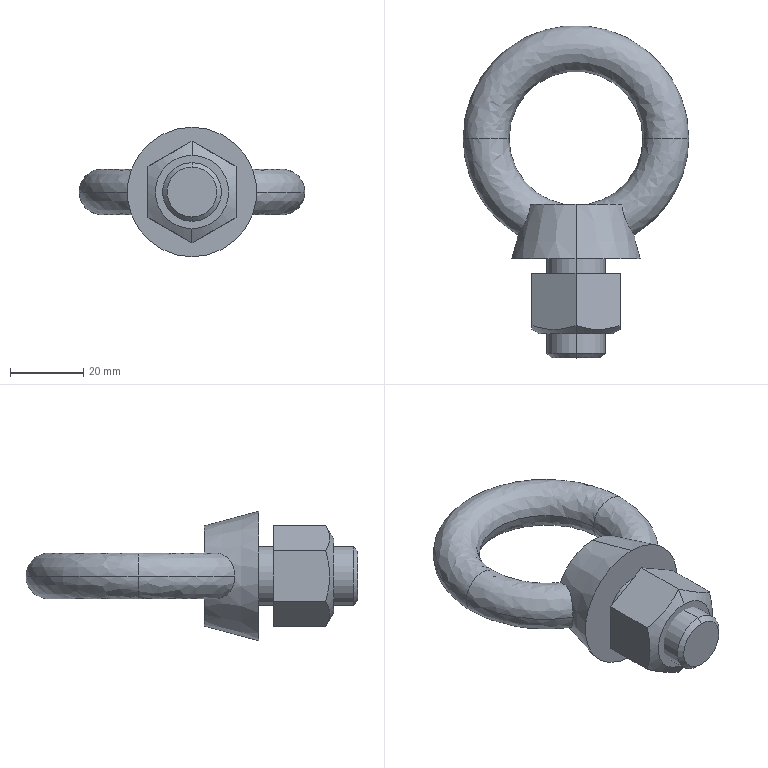Part | STEP file | M16-Lifting eye | 2 solids | 31 faces | box 61.5 x 90.6 x 35.3 mm | volume 37230 mm3 | plane 11 | cone 10 | spline 6 | cylinder 4 | commonest cylinder face diameters 16 x4
STEP:
#1=CARTESIAN_POINT('',(18.25,36.85,0.));
#2=VERTEX_POINT('',#1);
#3=CARTESIAN_POINT('',(3.295,18.9,0.));
#4=VERTEX_POINT('',#3);
#5=CARTESIAN_POINT('',(0.,36.85,0.));
#6=DIRECTION('',(0.,0.,-1.));
#7=DIRECTION('',(-1.,0.,0.));
#8=AXIS2_PLACEMENT_3D('',#5,#6,#7);
#9=CIRCLE('',#8,18.25);
#10=EDGE_CURVE('',#2,#4,#9,.T.);
#11=ORIENTED_EDGE('',*,*,#10,.F.);
#12=CARTESIAN_POINT('',(30.75,36.85,0.));
#13=VERTEX_POINT('',#12);
#14=CARTESIAN_POINT('',(24.5,36.85,0.));
#15=DIRECTION('',(0.,-1.,0.));
#16=DIRECTION('',(1.,0.,0.));
#17=AXIS2_PLACEMENT_3D('',#14,#15,#16);
#18=CIRCLE('',#17,6.25);
#19=EDGE_CURVE('',#2,#13,#18,.T.);
#20=ORIENTED_EDGE('',*,*,#19,.T.);
#21=CARTESIAN_POINT('',(15.9,10.53,0.));
#22=VERTEX_POINT('',#21);
#23=CARTESIAN_POINT('',(0.,36.85,0.));
#24=DIRECTION('',(0.,0.,-1.));
#25=DIRECTION('',(-1.,0.,0.));
#26=AXIS2_PLACEMENT_3D('',#23,#24,#25);
#27=CIRCLE('',#26,30.75);
#28=EDGE_CURVE('',#13,#22,#27,.T.);
#29=ORIENTED_EDGE('',*,*,#28,.T.);
#30=CARTESIAN_POINT('',(12.433,18.9,-5.653));
#31=VERTEX_POINT('',#30);
#32=CARTESIAN_POINT('',(15.9,10.53,0.));
#33=CARTESIAN_POINT('',(15.9,10.53,-0.5391));
#34=CARTESIAN_POINT('',(15.858,10.585,-1.067));
#35=CARTESIAN_POINT('',(15.737,10.748,-1.841));
#36=CARTESIAN_POINT('',(15.686,10.817,-2.098));
#37=CARTESIAN_POINT('',(15.567,10.98,-2.594));
#38=CARTESIAN_POINT('',(15.5,11.074,-2.833));
#39=CARTESIAN_POINT('',(15.349,11.288,-3.296));
#40=CARTESIAN_POINT('',(15.266,11.407,-3.52));
#41=CARTESIAN_POINT('',(15.087,11.673,-3.95));
#42=CARTESIAN_POINT('',(14.991,11.82,-4.155));
#43=CARTESIAN_POINT('',(14.792,12.132,-4.538));
#44=CARTESIAN_POINT('',(14.689,12.3,-4.717));
#45=CARTESIAN_POINT('',(14.476,12.657,-5.049));
#46=CARTESIAN_POINT('',(14.367,12.848,-5.203));
#47=CARTESIAN_POINT('',(14.037,13.454,-5.622));
#48=CARTESIAN_POINT('',(13.82,13.889,-5.836));
#49=CARTESIAN_POINT('',(13.514,14.594,-6.064));
#50=CARTESIAN_POINT('',(13.414,14.839,-6.124));
#51=CARTESIAN_POINT('',(13.229,15.333,-6.209));
#52=CARTESIAN_POINT('',(13.142,15.584,-6.235));
#53=CARTESIAN_POINT('',(12.902,16.344,-6.265));
#54=CARTESIAN_POINT('',(12.767,16.87,-6.22));
#55=CARTESIAN_POINT('',(12.56,17.896,-6.017));
#56=CARTESIAN_POINT('',(12.485,18.405,-5.859));
#57=CARTESIAN_POINT('',(12.433,18.9,-5.653));
#58=B_SPLINE_CURVE_WITH_KNOTS('',3,(#32,#33,#34,#35,#36,#37,#38,#39,#40,#41,#42,#43,#44,#45,#46,#47,#48,#49,#50,#51,#52,#53,#54,#55,#56,#57),.UNSPECIFIED.,.F.,.F.,(4,2,2,2,2,2,2,2,2,2,2,2,4),(0.01277,0.01436,0.01516,0.01595,0.01675,0.01755,0.01834,0.01914,0.02074,0.02153,0.02233,0.02392,0.02552),.UNSPECIFIED.);
#59=EDGE_CURVE('',#22,#31,#58,.T.);
#60=ORIENTED_EDGE('',*,*,#59,.T.);
#61=CARTESIAN_POINT('',(12.433,18.9,-5.653));
#62=CARTESIAN_POINT('',(11.533,18.9,-5.412));
#63=CARTESIAN_POINT('',(10.661,18.9,-5.112));
#64=CARTESIAN_POINT('',(8.96,18.9,-4.419));
#65=CARTESIAN_POINT('',(8.131,18.9,-4.028));
#66=CARTESIAN_POINT('',(6.917,18.9,-3.375));
#67=CARTESIAN_POINT('',(6.518,18.9,-3.147));
#68=CARTESIAN_POINT('',(5.731,18.9,-2.663));
#69=CARTESIAN_POINT('',(5.343,18.9,-2.408));
#70=CARTESIAN_POINT('',(4.78,18.9,-1.994));
#71=CARTESIAN_POINT('',(4.596,18.9,-1.851));
#72=CARTESIAN_POINT('',(4.24,18.9,-1.55));
#73=CARTESIAN_POINT('',(4.068,18.9,-1.392));
#74=CARTESIAN_POINT('',(3.751,18.9,-1.054));
#75=CARTESIAN_POINT('',(3.606,18.9,-0.8751));
#76=CARTESIAN_POINT('',(3.433,18.9,-0.5704));
#77=CARTESIAN_POINT('',(3.383,18.9,-0.4611));
#78=CARTESIAN_POINT('',(3.315,18.9,-0.2364));
#79=CARTESIAN_POINT('',(3.295,18.9,-0.1176));
#80=CARTESIAN_POINT('',(3.295,18.9,0.));
#81=B_SPLINE_CURVE_WITH_KNOTS('',3,(#61,#62,#63,#64,#65,#66,#67,#68,#69,#70,#71,#72,#73,#74,#75,#76,#77,#78,#79,#80),.UNSPECIFIED.,.F.,.F.,(4,2,2,2,2,2,2,2,2,4),(0.,0.002751,0.005503,0.006878,0.008254,0.008942,0.00963,0.01032,0.01066,0.01101),.UNSPECIFIED.);
#82=EDGE_CURVE('',#31,#4,#81,.T.);
#83=ORIENTED_EDGE('',*,*,#82,.T.);
#84=EDGE_LOOP('',(#11,#20,#29,#60,#83));
#85=FACE_OUTER_BOUND('',#84,.T.);
#86=CARTESIAN_POINT('',(18.25,36.85,0.));
#87=CARTESIAN_POINT('',(18.25,27.574,0.));
#88=CARTESIAN_POINT('',(12.283,20.472,0.));
#89=CARTESIAN_POINT('',(3.146,18.873,0.));
#90=CARTESIAN_POINT('',(18.25,36.85,-12.5));
#91=CARTESIAN_POINT('',(18.25,27.574,-12.5));
#92=CARTESIAN_POINT('',(12.283,20.472,-12.5));
#93=CARTESIAN_POINT('',(3.146,18.873,-12.5));
#94=CARTESIAN_POINT('',(30.75,36.85,-12.5));
#95=CARTESIAN_POINT('',(30.75,21.221,-12.5));
#96=CARTESIAN_POINT('',(20.696,9.254,-12.5));
#97=CARTESIAN_POINT('',(5.3,6.56,-12.5));
#98=CARTESIAN_POINT('',(30.75,36.85,0.));
#99=CARTESIAN_POINT('',(30.75,21.221,0.));
#100=CARTESIAN_POINT('',(20.696,9.254,0.));
#101=CARTESIAN_POINT('',(5.3,6.56,0.));
#102=(BOUNDED_SURFACE()B_SPLINE_SURFACE(3,3,((#86,#87,#88,#89),(#90,#91,#92,#93),(#94,#95,#96,#97),(#98,#99,#100,#101)),.UNSPECIFIED.,.F.,.F.,.T.)B_SPLINE_SURFACE_WITH_KNOTS((4,4),(4,4),(0.,1.),(0.,1.),.UNSPECIFIED.)GEOMETRIC_REPRESENTATION_ITEM()RATIONAL_B_SPLINE_SURFACE(((1.,0.8438,0.8438,1.),(0.3333,0.2813,0.2813,0.3333),(0.3333,0.2813,0.2813,0.3333),(1.,0.8438,0.8438,1.)))REPRESENTATION_ITEM('')SURFACE());
#103=ADVANCED_FACE('',(#85),#102,.T.);
#104=ORIENTED_EDGE('',*,*,#19,.F.);
#105=CARTESIAN_POINT('',(-18.25,36.85,0.));
#106=VERTEX_POINT('',#105);
#107=CARTESIAN_POINT('',(0.,36.85,0.));
#108=DIRECTION('',(0.,0.,-1.));
#109=DIRECTION('',(-1.,0.,0.));
#110=AXIS2_PLACEMENT_3D('',#107,#108,#109);
#111=CIRCLE('',#110,18.25);
#112=EDGE_CURVE('',#106,#2,#111,.T.);
#113=ORIENTED_EDGE('',*,*,#112,.F.);
#114=CARTESIAN_POINT('',(-30.75,36.85,0.));
#115=VERTEX_POINT('',#114);
#116=CARTESIAN_POINT('',(-24.5,36.85,0.));
#117=DIRECTION('',(0.,1.,0.));
#118=DIRECTION('',(-1.,0.,0.));
#119=AXIS2_PLACEMENT_3D('',#116,#117,#118);
#120=CIRCLE('',#119,6.25);
#121=EDGE_CURVE('',#106,#115,#120,.T.);
#122=ORIENTED_EDGE('',*,*,#121,.T.);
#123=CARTESIAN_POINT('',(0.,36.85,0.));
#124=DIRECTION('',(0.,0.,-1.));
#125=DIRECTION('',(-1.,0.,0.));
#126=AXIS2_PLACEMENT_3D('',#123,#124,#125);
#127=CIRCLE('',#126,30.75);
#128=EDGE_CURVE('',#115,#13,#127,.T.);
#129=ORIENTED_EDGE('',*,*,#128,.T.);
#130=EDGE_LOOP('',(#104,#113,#122,#129));
#131=FACE_OUTER_BOUND('',#130,.T.);
#132=CARTESIAN_POINT('',(-18.25,36.85,0.));
#133=CARTESIAN_POINT('',(-18.25,73.35,0.));
#134=CARTESIAN_POINT('',(18.25,73.35,0.));
#135=CARTESIAN_POINT('',(18.25,36.85,0.));
#136=CARTESIAN_POINT('',(-18.25,36.85,-12.5));
#137=CARTESIAN_POINT('',(-18.25,73.35,-12.5));
#138=CARTESIAN_POINT('',(18.25,73.35,-12.5));
#139=CARTESIAN_POINT('',(18.25,36.85,-12.5));
#140=CARTESIAN_POINT('',(-30.75,36.85,-12.5));
#141=CARTESIAN_POINT('',(-30.75,98.35,-12.5));
#142=CARTESIAN_POINT('',(30.75,98.35,-12.5));
#143=CARTESIAN_POINT('',(30.75,36.85,-12.5));
#144=CARTESIAN_POINT('',(-30.75,36.85,0.));
#145=CARTESIAN_POINT('',(-30.75,98.35,0.));
#146=CARTESIAN_POINT('',(30.75,98.35,0.));
#147=CARTESIAN_POINT('',(30.75,36.85,0.));
#148=(BOUNDED_SURFACE()B_SPLINE_SURFACE(3,3,((#132,#133,#134,#135),(#136,#137,#138,#139),(#140,#141,#142,#143),(#144,#145,#146,#147)),.UNSPECIFIED.,.F.,.F.,.F.)B_SPLINE_SURFACE_WITH_KNOTS((4,4),(4,4),(0.,1.),(0.,1.),.UNSPECIFIED.)GEOMETRIC_REPRESENTATION_ITEM()RATIONAL_B_SPLINE_SURFACE(((1.,0.3333,0.3333,1.),(0.3333,0.1111,0.1111,0.3333),(0.3333,0.1111,0.1111,0.3333),(1.,0.3333,0.3333,1.)))REPRESENTATION_ITEM('')SURFACE());
#149=ADVANCED_FACE('',(#131),#148,.T.);
#150=ORIENTED_EDGE('',*,*,#28,.F.);
#151=CARTESIAN_POINT('',(24.5,36.85,0.));
#152=DIRECTION('',(0.,-1.,0.));
#153=DIRECTION('',(1.,0.,0.));
#154=AXIS2_PLACEMENT_3D('',#151,#152,#153);
#155=CIRCLE('',#154,6.25);
#156=EDGE_CURVE('',#13,#2,#155,.T.);
#157=ORIENTED_EDGE('',*,*,#156,.T.);
#158=ORIENTED_EDGE('',*,*,#10,.T.);
#159=CARTESIAN_POINT('',(12.433,18.9,5.653));
#160=VERTEX_POINT('',#159);
#161=CARTESIAN_POINT('',(3.295,18.9,0.));
#162=CARTESIAN_POINT('',(3.295,18.9,0.1168));
#163=CARTESIAN_POINT('',(3.314,18.9,0.2323));
#164=CARTESIAN_POINT('',(3.382,18.9,0.4583));
#165=CARTESIAN_POINT('',(3.43,18.9,0.5644));
#166=CARTESIAN_POINT('',(3.544,18.9,0.7679));
#167=CARTESIAN_POINT('',(3.611,18.9,0.8656));
#168=CARTESIAN_POINT('',(3.754,18.9,1.05));
#169=CARTESIAN_POINT('',(3.83,18.9,1.138));
#170=CARTESIAN_POINT('',(4.067,18.9,1.391));
#171=CARTESIAN_POINT('',(4.238,18.9,1.547));
#172=CARTESIAN_POINT('',(4.592,18.9,1.848));
#173=CARTESIAN_POINT('',(4.776,18.9,1.991));
#174=CARTESIAN_POINT('',(5.335,18.9,2.402));
#175=CARTESIAN_POINT('',(5.72,18.9,2.656));
#176=CARTESIAN_POINT('',(6.503,18.9,3.138));
#177=CARTESIAN_POINT('',(6.902,18.9,3.367));
#178=CARTESIAN_POINT('',(8.116,18.9,4.02));
#179=CARTESIAN_POINT('',(8.95,18.9,4.415));
#180=CARTESIAN_POINT('',(10.664,18.9,5.113));
#181=CARTESIAN_POINT('',(11.538,18.9,5.413));
#182=CARTESIAN_POINT('',(12.433,18.9,5.653));
#183=B_SPLINE_CURVE_WITH_KNOTS('',3,(#161,#162,#163,#164,#165,#166,#167,#168,#169,#170,#171,#172,#173,#174,#175,#176,#177,#178,#179,#180,#181,#182),.UNSPECIFIED.,.F.,.F.,(4,2,2,2,2,2,2,2,2,2,4),(0.01101,0.01135,0.01169,0.01203,0.01237,0.01306,0.01374,0.01511,0.01647,0.0192,0.02194),.UNSPECIFIED.);
#184=EDGE_CURVE('',#4,#160,#183,.T.);
#185=ORIENTED_EDGE('',*,*,#184,.T.);
#186=CARTESIAN_POINT('',(12.433,18.9,5.653));
#187=CARTESIAN_POINT('',(12.485,18.405,5.859));
#188=CARTESIAN_POINT('',(12.559,17.901,6.015));
#189=CARTESIAN_POINT('',(12.714,17.132,6.168));
#190=CARTESIAN_POINT('',(12.773,16.872,6.205));
#191=CARTESIAN_POINT('',(12.907,16.353,6.249));
#192=CARTESIAN_POINT('',(12.98,16.097,6.255));
#193=CARTESIAN_POINT('',(13.139,15.591,6.236));
#194=CARTESIAN_POINT('',(13.226,15.342,6.21));
#195=CARTESIAN_POINT('',(13.41,14.85,6.126));
#196=CARTESIAN_POINT('',(13.509,14.605,6.067));
#197=CARTESIAN_POINT('',(13.817,13.896,5.839));
#198=CARTESIAN_POINT('',(14.033,13.46,5.625));
#199=CARTESIAN_POINT('',(14.363,12.855,5.209));
#200=CARTESIAN_POINT('',(14.473,12.663,5.054));
#201=CARTESIAN_POINT('',(14.686,12.303,4.721));
#202=CARTESIAN_POINT('',(14.79,12.136,4.542));
#203=CARTESIAN_POINT('',(14.989,11.822,4.159));
#204=CARTESIAN_POINT('',(15.086,11.676,3.953));
#205=CARTESIAN_POINT('',(15.265,11.409,3.523));
#206=CARTESIAN_POINT('',(15.348,11.289,3.299));
#207=CARTESIAN_POINT('',(15.499,11.075,2.836));
#208=CARTESIAN_POINT('',(15.567,10.981,2.596));
#209=CARTESIAN_POINT('',(15.685,10.817,2.099));
#210=CARTESIAN_POINT('',(15.736,10.748,1.842));
#211=CARTESIAN_POINT('',(15.858,10.585,1.068));
#212=CARTESIAN_POINT('',(15.9,10.53,0.5397));
#213=CARTESIAN_POINT('',(15.9,10.53,0.));
#214=B_SPLINE_CURVE_WITH_KNOTS('',3,(#186,#187,#188,#189,#190,#191,#192,#193,#194,#195,#196,#197,#198,#199,#200,#201,#202,#203,#204,#205,#206,#207,#208,#209,#210,#211,#212,#213),.UNSPECIFIED.,.F.,.F.,(4,2,2,2,2,2,2,2,2,2,2,2,2,4),(0.,0.001596,0.002393,0.003191,0.003989,0.004787,0.006383,0.00718,0.007978,0.008776,0.009574,0.01037,0.01117,0.01277),.UNSPECIFIED.);
#215=EDGE_CURVE('',#160,#22,#214,.T.);
#216=ORIENTED_EDGE('',*,*,#215,.T.);
#217=EDGE_LOOP('',(#150,#157,#158,#185,#216));
#218=FACE_OUTER_BOUND('',#217,.T.);
#219=CARTESIAN_POINT('',(30.75,36.85,0.));
#220=CARTESIAN_POINT('',(30.75,21.221,0.));
#221=CARTESIAN_POINT('',(20.696,9.254,0.));
#222=CARTESIAN_POINT('',(5.3,6.56,0.));
#223=CARTESIAN_POINT('',(30.75,36.85,12.5));
#224=CARTESIAN_POINT('',(30.75,21.221,12.5));
#225=CARTESIAN_POINT('',(20.696,9.254,12.5));
#226=CARTESIAN_POINT('',(5.3,6.56,12.5));
#227=CARTESIAN_POINT('',(18.25,36.85,12.5));
#228=CARTESIAN_POINT('',(18.25,27.574,12.5));
#229=CARTESIAN_POINT('',(12.283,20.472,12.5));
#230=CARTESIAN_POINT('',(3.146,18.873,12.5));
#231=CARTESIAN_POINT('',(18.25,36.85,0.));
#232=CARTESIAN_POINT('',(18.25,27.574,0.));
#233=CARTESIAN_POINT('',(12.283,20.472,0.));
#234=CARTESIAN_POINT('',(3.146,18.873,0.));
#235=(BOUNDED_SURFACE()B_SPLINE_SURFACE(3,3,((#219,#220,#221,#222),(#223,#224,#225,#226),(#227,#228,#229,#230),(#231,#232,#233,#234)),.UNSPECIFIED.,.F.,.F.,.T.)B_SPLINE_SURFACE_WITH_KNOTS((4,4),(4,4),(0.,1.),(0.,1.),.UNSPECIFIED.)GEOMETRIC_REPRESENTATION_ITEM()RATIONAL_B_SPLINE_SURFACE(((1.,0.8438,0.8438,1.),(0.3333,0.2813,0.2813,0.3333),(0.3333,0.2813,0.2813,0.3333),(1.,0.8438,0.8438,1.)))REPRESENTATION_ITEM('')SURFACE());
#236=ADVANCED_FACE('',(#218),#235,.T.);
#237=ORIENTED_EDGE('',*,*,#156,.F.);
#238=ORIENTED_EDGE('',*,*,#128,.F.);
#239=CARTESIAN_POINT('',(-24.5,36.85,0.));
#240=DIRECTION('',(0.,1.,0.));
#241=DIRECTION('',(-1.,0.,0.));
#242=AXIS2_PLACEMENT_3D('',#239,#240,#241);
#243=CIRCLE('',#242,6.25);
#244=EDGE_CURVE('',#115,#106,#243,.T.);
#245=ORIENTED_EDGE('',*,*,#244,.T.);
#246=ORIENTED_EDGE('',*,*,#112,.T.);
#247=EDGE_LOOP('',(#237,#238,#245,#246));
#248=FACE_OUTER_BOUND('',#247,.T.);
#249=CARTESIAN_POINT('',(-30.75,36.85,0.));
#250=CARTESIAN_POINT('',(-30.75,98.35,0.));
#251=CARTESIAN_POINT('',(30.75,98.35,0.));
#252=CARTESIAN_POINT('',(30.75,36.85,0.));
#253=CARTESIAN_POINT('',(-30.75,36.85,12.5));
#254=CARTESIAN_POINT('',(-30.75,98.35,12.5));
#255=CARTESIAN_POINT('',(30.75,98.35,12.5));
#256=CARTESIAN_POINT('',(30.75,36.85,12.5));
#257=CARTESIAN_POINT('',(-18.25,36.85,12.5));
#258=CARTESIAN_POINT('',(-18.25,73.35,12.5));
#259=CARTESIAN_POINT('',(18.25,73.35,12.5));
#260=CARTESIAN_POINT('',(18.25,36.85,12.5));
#261=CARTESIAN_POINT('',(-18.25,36.85,0.));
#262=CARTESIAN_POINT('',(-18.25,73.35,0.));
#263=CARTESIAN_POINT('',(18.25,73.35,0.));
#264=CARTESIAN_POINT('',(18.25,36.85,0.));
#265=(BOUNDED_SURFACE()B_SPLINE_SURFACE(3,3,((#249,#250,#251,#252),(#253,#254,#255,#256),(#257,#258,#259,#260),(#261,#262,#263,#264)),.UNSPECIFIED.,.F.,.F.,.T.)B_SPLINE_SURFACE_WITH_KNOTS((4,4),(4,4),(0.,1.),(0.,1.),.UNSPECIFIED.)GEOMETRIC_REPRESENTATION_ITEM()RATIONAL_B_SPLINE_SURFACE(((1.,0.3333,0.3333,1.),(0.3333,0.1111,0.1111,0.3333),(0.3333,0.1111,0.1111,0.3333),(1.,0.3333,0.3333,1.)))REPRESENTATION_ITEM('')SURFACE());
#266=ADVANCED_FACE('',(#248),#265,.T.);
#267=ORIENTED_EDGE('',*,*,#244,.F.);
#268=CARTESIAN_POINT('',(-15.9,10.53,0.));
#269=VERTEX_POINT('',#268);
#270=CARTESIAN_POINT('',(0.,36.85,0.));
#271=DIRECTION('',(0.,0.,-1.));
#272=DIRECTION('',(-1.,0.,0.));
#273=AXIS2_PLACEMENT_3D('',#270,#271,#272);
#274=CIRCLE('',#273,30.75);
#275=EDGE_CURVE('',#269,#115,#274,.T.);
#276=ORIENTED_EDGE('',*,*,#275,.F.);
#277=CARTESIAN_POINT('',(-12.433,18.9,5.653));
#278=VERTEX_POINT('',#277);
#279=CARTESIAN_POINT('',(-15.9,10.53,0.));
#280=CARTESIAN_POINT('',(-15.9,10.53,0.5391));
#281=CARTESIAN_POINT('',(-15.858,10.585,1.067));
#282=CARTESIAN_POINT('',(-15.737,10.748,1.841));
#283=CARTESIAN_POINT('',(-15.686,10.817,2.098));
#284=CARTESIAN_POINT('',(-15.567,10.98,2.594));
#285=CARTESIAN_POINT('',(-15.5,11.074,2.833));
#286=CARTESIAN_POINT('',(-15.349,11.288,3.296));
#287=CARTESIAN_POINT('',(-15.266,11.407,3.52));
#288=CARTESIAN_POINT('',(-15.087,11.673,3.95));
#289=CARTESIAN_POINT('',(-14.991,11.82,4.155));
#290=CARTESIAN_POINT('',(-14.792,12.132,4.538));
#291=CARTESIAN_POINT('',(-14.689,12.3,4.717));
#292=CARTESIAN_POINT('',(-14.476,12.657,5.049));
#293=CARTESIAN_POINT('',(-14.367,12.848,5.203));
#294=CARTESIAN_POINT('',(-14.037,13.454,5.622));
#295=CARTESIAN_POINT('',(-13.82,13.889,5.836));
#296=CARTESIAN_POINT('',(-13.514,14.594,6.064));
#297=CARTESIAN_POINT('',(-13.414,14.839,6.124));
#298=CARTESIAN_POINT('',(-13.229,15.333,6.209));
#299=CARTESIAN_POINT('',(-13.142,15.584,6.235));
#300=CARTESIAN_POINT('',(-12.902,16.344,6.265));
#301=CARTESIAN_POINT('',(-12.767,16.87,6.22));
#302=CARTESIAN_POINT('',(-12.56,17.896,6.017));
#303=CARTESIAN_POINT('',(-12.485,18.405,5.859));
#304=CARTESIAN_POINT('',(-12.433,18.9,5.653));
#305=B_SPLINE_CURVE_WITH_KNOTS('',3,(#279,#280,#281,#282,#283,#284,#285,#286,#287,#288,#289,#290,#291,#292,#293,#294,#295,#296,#297,#298,#299,#300,#301,#302,#303,#304),.UNSPECIFIED.,.F.,.F.,(4,2,2,2,2,2,2,2,2,2,2,2,4),(0.01277,0.01436,0.01516,0.01595,0.01675,0.01755,0.01834,0.01914,0.02074,0.02153,0.02233,0.02392,0.02552),.UNSPECIFIED.);
#306=EDGE_CURVE('',#269,#278,#305,.T.);
#307=ORIENTED_EDGE('',*,*,#306,.T.);
#308=CARTESIAN_POINT('',(-3.295,18.9,0.));
#309=VERTEX_POINT('',#308);
#310=CARTESIAN_POINT('',(-12.433,18.9,5.653));
#311=CARTESIAN_POINT('',(-11.533,18.9,5.412));
#312=CARTESIAN_POINT('',(-10.661,18.9,5.112));
#313=CARTESIAN_POINT('',(-8.96,18.9,4.419));
#314=CARTESIAN_POINT('',(-8.131,18.9,4.028));
#315=CARTESIAN_POINT('',(-6.917,18.9,3.375));
#316=CARTESIAN_POINT('',(-6.518,18.9,3.147));
#317=CARTESIAN_POINT('',(-5.731,18.9,2.663));
#318=CARTESIAN_POINT('',(-5.343,18.9,2.408));
#319=CARTESIAN_POINT('',(-4.78,18.9,1.994));
#320=CARTESIAN_POINT('',(-4.596,18.9,1.851));
#321=CARTESIAN_POINT('',(-4.24,18.9,1.55));
#322=CARTESIAN_POINT('',(-4.068,18.9,1.392));
#323=CARTESIAN_POINT('',(-3.751,18.9,1.054));
#324=CARTESIAN_POINT('',(-3.606,18.9,0.8751));
#325=CARTESIAN_POINT('',(-3.433,18.9,0.5704));
#326=CARTESIAN_POINT('',(-3.383,18.9,0.4611));
#327=CARTESIAN_POINT('',(-3.315,18.9,0.2364));
#328=CARTESIAN_POINT('',(-3.295,18.9,0.1176));
#329=CARTESIAN_POINT('',(-3.295,18.9,0.));
#330=B_SPLINE_CURVE_WITH_KNOTS('',3,(#310,#311,#312,#313,#314,#315,#316,#317,#318,#319,#320,#321,#322,#323,#324,#325,#326,#327,#328,#329),.UNSPECIFIED.,.F.,.F.,(4,2,2,2,2,2,2,2,2,4),(0.,0.002751,0.005503,0.006878,0.008254,0.008942,0.00963,0.01032,0.01066,0.01101),.UNSPECIFIED.);
#331=EDGE_CURVE('',#278,#309,#330,.T.);
#332=ORIENTED_EDGE('',*,*,#331,.T.);
#333=CARTESIAN_POINT('',(0.,36.85,0.));
#334=DIRECTION('',(0.,0.,-1.));
#335=DIRECTION('',(-1.,0.,0.));
#336=AXIS2_PLACEMENT_3D('',#333,#334,#335);
#337=CIRCLE('',#336,18.25);
#338=EDGE_CURVE('',#309,#106,#337,.T.);
#339=ORIENTED_EDGE('',*,*,#338,.T.);
#340=EDGE_LOOP('',(#267,#276,#307,#332,#339));
#341=FACE_OUTER_BOUND('',#340,.T.);
#342=CARTESIAN_POINT('',(-5.3,6.56,0.));
#343=CARTESIAN_POINT('',(-20.696,9.254,0.));
#344=CARTESIAN_POINT('',(-30.75,21.221,0.));
#345=CARTESIAN_POINT('',(-30.75,36.85,0.));
#346=CARTESIAN_POINT('',(-5.3,6.56,12.5));
#347=CARTESIAN_POINT('',(-20.696,9.254,12.5));
#348=CARTESIAN_POINT('',(-30.75,21.221,12.5));
#349=CARTESIAN_POINT('',(-30.75,36.85,12.5));
#350=CARTESIAN_POINT('',(-3.146,18.873,12.5));
#351=CARTESIAN_POINT('',(-12.283,20.472,12.5));
#352=CARTESIAN_POINT('',(-18.25,27.574,12.5));
#353=CARTESIAN_POINT('',(-18.25,36.85,12.5));
#354=CARTESIAN_POINT('',(-3.146,18.873,0.));
#355=CARTESIAN_POINT('',(-12.283,20.472,0.));
#356=CARTESIAN_POINT('',(-18.25,27.574,0.));
#357=CARTESIAN_POINT('',(-18.25,36.85,0.));
#358=(BOUNDED_SURFACE()B_SPLINE_SURFACE(3,3,((#342,#343,#344,#345),(#346,#347,#348,#349),(#350,#351,#352,#353),(#354,#355,#356,#357)),.UNSPECIFIED.,.F.,.F.,.T.)B_SPLINE_SURFACE_WITH_KNOTS((4,4),(4,4),(0.,1.),(0.,1.),.UNSPECIFIED.)GEOMETRIC_REPRESENTATION_ITEM()RATIONAL_B_SPLINE_SURFACE(((1.,0.8438,0.8438,1.),(0.3333,0.2813,0.2813,0.3333),(0.3333,0.2813,0.2813,0.3333),(1.,0.8438,0.8438,1.)))REPRESENTATION_ITEM('')SURFACE());
#359=ADVANCED_FACE('',(#341),#358,.T.);
#360=CARTESIAN_POINT('',(0.,18.9,13.658));
#361=VERTEX_POINT('',#360);
#362=CARTESIAN_POINT('',(0.,18.9,0.));
#363=DIRECTION('',(0.,-1.,0.));
#364=DIRECTION('',(0.,0.,-1.));
#365=AXIS2_PLACEMENT_3D('',#362,#363,#364);
#366=CIRCLE('',#365,13.658);
#367=EDGE_CURVE('',#160,#361,#366,.T.);
#368=ORIENTED_EDGE('',*,*,#367,.T.);
#369=CARTESIAN_POINT('',(0.,4.,17.65));
#370=VERTEX_POINT('',#369);
#371=CARTESIAN_POINT('',(0.,4.,17.65));
#372=DIRECTION('',(0.,-0.9659,0.2588));
#373=VECTOR('',#372,1000.);
#374=LINE('',#371,#373);
#375=EDGE_CURVE('',#361,#370,#374,.T.);
#376=ORIENTED_EDGE('',*,*,#375,.T.);
#377=CARTESIAN_POINT('',(0.,4.,-17.65));
#378=VERTEX_POINT('',#377);
#379=CARTESIAN_POINT('',(0.,4.,0.));
#380=DIRECTION('',(0.,1.,0.));
#381=DIRECTION('',(0.,0.,-1.));
#382=AXIS2_PLACEMENT_3D('',#379,#380,#381);
#383=CIRCLE('',#382,17.65);
#384=EDGE_CURVE('',#370,#378,#383,.T.);
#385=ORIENTED_EDGE('',*,*,#384,.T.);
#386=CARTESIAN_POINT('',(0.,18.9,-13.658));
#387=VERTEX_POINT('',#386);
#388=CARTESIAN_POINT('',(0.,4.,-17.65));
#389=DIRECTION('',(0.,-0.9659,-0.2588));
#390=VECTOR('',#389,1000.);
#391=LINE('',#388,#390);
#392=EDGE_CURVE('',#387,#378,#391,.T.);
#393=ORIENTED_EDGE('',*,*,#392,.F.);
#394=CARTESIAN_POINT('',(0.,18.9,0.));
#395=DIRECTION('',(0.,-1.,0.));
#396=DIRECTION('',(0.,0.,-1.));
#397=AXIS2_PLACEMENT_3D('',#394,#395,#396);
#398=CIRCLE('',#397,13.658);
#399=EDGE_CURVE('',#387,#31,#398,.T.);
#400=ORIENTED_EDGE('',*,*,#399,.T.);
#401=ORIENTED_EDGE('',*,*,#59,.F.);
#402=ORIENTED_EDGE('',*,*,#215,.F.);
#403=EDGE_LOOP('',(#368,#376,#385,#393,#400,#401,#402));
#404=FACE_OUTER_BOUND('',#403,.T.);
#405=CARTESIAN_POINT('',(0.,4.,0.));
#406=DIRECTION('',(0.,-1.,0.));
#407=DIRECTION('',(0.,0.,-1.));
#408=AXIS2_PLACEMENT_3D('',#405,#406,#407);
#409=CONICAL_SURFACE('',#408,17.65,0.2618);
#410=ADVANCED_FACE('',(#404),#409,.T.);
#411=CARTESIAN_POINT('',(0.,4.,-8.));
#412=VERTEX_POINT('',#411);
#413=CARTESIAN_POINT('',(0.,4.,8.));
#414=VERTEX_POINT('',#413);
#415=CARTESIAN_POINT('',(0.,4.,0.));
#416=DIRECTION('',(0.,-1.,0.));
#417=DIRECTION('',(0.,0.,-1.));
#418=AXIS2_PLACEMENT_3D('',#415,#416,#417);
#419=CIRCLE('',#418,8.);
#420=EDGE_CURVE('',#412,#414,#419,.T.);
#421=ORIENTED_EDGE('',*,*,#420,.T.);
#422=CARTESIAN_POINT('',(0.,-21.773,8.));
#423=VERTEX_POINT('',#422);
#424=CARTESIAN_POINT('',(0.,18.9,8.));
#425=DIRECTION('',(0.,-1.,0.));
#426=VECTOR('',#425,1000.);
#427=LINE('',#424,#426);
#428=EDGE_CURVE('',#414,#423,#427,.T.);
#429=ORIENTED_EDGE('',*,*,#428,.T.);
#430=CARTESIAN_POINT('',(0.,-21.773,-8.));
#431=VERTEX_POINT('',#430);
#432=CARTESIAN_POINT('',(0.,-21.773,0.));
#433=DIRECTION('',(0.,1.,0.));
#434=DIRECTION('',(0.,0.,-1.));
#435=AXIS2_PLACEMENT_3D('',#432,#433,#434);
#436=CIRCLE('',#435,8.);
#437=EDGE_CURVE('',#423,#431,#436,.T.);
#438=ORIENTED_EDGE('',*,*,#437,.T.);
#439=CARTESIAN_POINT('',(0.,18.9,-8.));
#440=DIRECTION('',(0.,-1.,0.));
#441=VECTOR('',#440,1000.);
#442=LINE('',#439,#441);
#443=EDGE_CURVE('',#412,#431,#442,.T.);
#444=ORIENTED_EDGE('',*,*,#443,.F.);
#445=EDGE_LOOP('',(#421,#429,#438,#444));
#446=FACE_OUTER_BOUND('',#445,.T.);
#447=CARTESIAN_POINT('',(0.,18.9,0.));
#448=DIRECTION('',(0.,-1.,0.));
#449=DIRECTION('',(0.,0.,-1.));
#450=AXIS2_PLACEMENT_3D('',#447,#448,#449);
#451=CYLINDRICAL_SURFACE('',#450,8.);
#452=ADVANCED_FACE('',(#446),#451,.T.);
#453=CARTESIAN_POINT('',(0.,-23.,6.773));
#454=VERTEX_POINT('',#453);
#455=CARTESIAN_POINT('',(0.,-23.,-6.773));
#456=VERTEX_POINT('',#455);
#457=CARTESIAN_POINT('',(0.,-23.,0.));
#458=DIRECTION('',(0.,1.,0.));
#459=DIRECTION('',(0.,0.,1.));
#460=AXIS2_PLACEMENT_3D('',#457,#458,#459);
#461=CIRCLE('',#460,6.773);
#462=EDGE_CURVE('',#454,#456,#461,.T.);
#463=ORIENTED_EDGE('',*,*,#462,.T.);
#464=CARTESIAN_POINT('',(0.,-21.773,-8.));
#465=DIRECTION('',(0.,0.7071,-0.7071));
#466=VECTOR('',#465,1000.);
#467=LINE('',#464,#466);
#468=EDGE_CURVE('',#456,#431,#467,.T.);
#469=ORIENTED_EDGE('',*,*,#468,.T.);
#470=ORIENTED_EDGE('',*,*,#437,.F.);
#471=CARTESIAN_POINT('',(0.,-21.773,8.));
#472=DIRECTION('',(0.,0.7071,0.7071));
#473=VECTOR('',#472,1000.);
#474=LINE('',#471,#473);
#475=EDGE_CURVE('',#454,#423,#474,.T.);
#476=ORIENTED_EDGE('',*,*,#475,.F.);
#477=EDGE_LOOP('',(#463,#469,#470,#476));
#478=FACE_OUTER_BOUND('',#477,.T.);
#479=CARTESIAN_POINT('',(0.,-21.773,0.));
#480=DIRECTION('',(0.,1.,0.));
#481=DIRECTION('',(0.,0.,1.));
#482=AXIS2_PLACEMENT_3D('',#479,#480,#481);
#483=CONICAL_SURFACE('',#482,8.,0.7854);
#484=ADVANCED_FACE('',(#478),#483,.T.);
#485=ORIENTED_EDGE('',*,*,#121,.F.);
#486=ORIENTED_EDGE('',*,*,#338,.F.);
#487=CARTESIAN_POINT('',(-12.433,18.9,-5.653));
#488=VERTEX_POINT('',#487);
#489=CARTESIAN_POINT('',(-3.295,18.9,0.));
#490=CARTESIAN_POINT('',(-3.295,18.9,-0.1168));
#491=CARTESIAN_POINT('',(-3.314,18.9,-0.2323));
#492=CARTESIAN_POINT('',(-3.382,18.9,-0.4583));
#493=CARTESIAN_POINT('',(-3.43,18.9,-0.5644));
#494=CARTESIAN_POINT('',(-3.544,18.9,-0.7679));
#495=CARTESIAN_POINT('',(-3.611,18.9,-0.8656));
#496=CARTESIAN_POINT('',(-3.754,18.9,-1.05));
#497=CARTESIAN_POINT('',(-3.83,18.9,-1.138));
#498=CARTESIAN_POINT('',(-4.067,18.9,-1.391));
#499=CARTESIAN_POINT('',(-4.238,18.9,-1.547));
#500=CARTESIAN_POINT('',(-4.592,18.9,-1.848));
#501=CARTESIAN_POINT('',(-4.776,18.9,-1.991));
#502=CARTESIAN_POINT('',(-5.335,18.9,-2.402));
#503=CARTESIAN_POINT('',(-5.72,18.9,-2.656));
#504=CARTESIAN_POINT('',(-6.503,18.9,-3.138));
#505=CARTESIAN_POINT('',(-6.902,18.9,-3.367));
#506=CARTESIAN_POINT('',(-8.116,18.9,-4.02));
#507=CARTESIAN_POINT('',(-8.95,18.9,-4.415));
#508=CARTESIAN_POINT('',(-10.664,18.9,-5.113));
#509=CARTESIAN_POINT('',(-11.538,18.9,-5.413));
#510=CARTESIAN_POINT('',(-12.433,18.9,-5.653));
#511=B_SPLINE_CURVE_WITH_KNOTS('',3,(#489,#490,#491,#492,#493,#494,#495,#496,#497,#498,#499,#500,#501,#502,#503,#504,#505,#506,#507,#508,#509,#510),.UNSPECIFIED.,.F.,.F.,(4,2,2,2,2,2,2,2,2,2,4),(0.01101,0.01135,0.01169,0.01203,0.01237,0.01306,0.01374,0.01511,0.01647,0.0192,0.02194),.UNSPECIFIED.);
#512=EDGE_CURVE('',#309,#488,#511,.T.);
#513=ORIENTED_EDGE('',*,*,#512,.T.);
#514=CARTESIAN_POINT('',(-12.433,18.9,-5.653));
#515=CARTESIAN_POINT('',(-12.485,18.405,-5.859));
#516=CARTESIAN_POINT('',(-12.559,17.901,-6.015));
#517=CARTESIAN_POINT('',(-12.714,17.132,-6.168));
#518=CARTESIAN_POINT('',(-12.773,16.872,-6.205));
#519=CARTESIAN_POINT('',(-12.907,16.353,-6.249));
#520=CARTESIAN_POINT('',(-12.98,16.097,-6.255));
#521=CARTESIAN_POINT('',(-13.139,15.591,-6.236));
#522=CARTESIAN_POINT('',(-13.226,15.342,-6.21));
#523=CARTESIAN_POINT('',(-13.41,14.85,-6.126));
#524=CARTESIAN_POINT('',(-13.509,14.605,-6.067));
#525=CARTESIAN_POINT('',(-13.817,13.896,-5.839));
#526=CARTESIAN_POINT('',(-14.033,13.46,-5.625));
#527=CARTESIAN_POINT('',(-14.363,12.855,-5.209));
#528=CARTESIAN_POINT('',(-14.473,12.663,-5.054));
#529=CARTESIAN_POINT('',(-14.686,12.303,-4.721));
#530=CARTESIAN_POINT('',(-14.79,12.136,-4.542));
#531=CARTESIAN_POINT('',(-14.989,11.822,-4.159));
#532=CARTESIAN_POINT('',(-15.086,11.676,-3.953));
#533=CARTESIAN_POINT('',(-15.265,11.409,-3.523));
#534=CARTESIAN_POINT('',(-15.348,11.289,-3.299));
#535=CARTESIAN_POINT('',(-15.499,11.075,-2.836));
#536=CARTESIAN_POINT('',(-15.567,10.981,-2.596));
#537=CARTESIAN_POINT('',(-15.685,10.817,-2.099));
#538=CARTESIAN_POINT('',(-15.736,10.748,-1.842));
#539=CARTESIAN_POINT('',(-15.858,10.585,-1.068));
#540=CARTESIAN_POINT('',(-15.9,10.53,-0.5397));
#541=CARTESIAN_POINT('',(-15.9,10.53,0.));
#542=B_SPLINE_CURVE_WITH_KNOTS('',3,(#514,#515,#516,#517,#518,#519,#520,#521,#522,#523,#524,#525,#526,#527,#528,#529,#530,#531,#532,#533,#534,#535,#536,#537,#538,#539,#540,#541),.UNSPECIFIED.,.F.,.F.,(4,2,2,2,2,2,2,2,2,2,2,2,2,4),(0.,0.001596,0.002393,0.003191,0.003989,0.004787,0.006383,0.00718,0.007978,0.008776,0.009574,0.01037,0.01117,0.01277),.UNSPECIFIED.);
#543=EDGE_CURVE('',#488,#269,#542,.T.);
#544=ORIENTED_EDGE('',*,*,#543,.T.);
#545=ORIENTED_EDGE('',*,*,#275,.T.);
#546=EDGE_LOOP('',(#485,#486,#513,#544,#545));
#547=FACE_OUTER_BOUND('',#546,.T.);
#548=CARTESIAN_POINT('',(-3.146,18.873,0.));
#549=CARTESIAN_POINT('',(-12.283,20.472,0.));
#550=CARTESIAN_POINT('',(-18.25,27.574,0.));
#551=CARTESIAN_POINT('',(-18.25,36.85,0.));
#552=CARTESIAN_POINT('',(-3.146,18.873,-12.5));
#553=CARTESIAN_POINT('',(-12.283,20.472,-12.5));
#554=CARTESIAN_POINT('',(-18.25,27.574,-12.5));
#555=CARTESIAN_POINT('',(-18.25,36.85,-12.5));
#556=CARTESIAN_POINT('',(-5.3,6.56,-12.5));
#557=CARTESIAN_POINT('',(-20.696,9.254,-12.5));
#558=CARTESIAN_POINT('',(-30.75,21.221,-12.5));
#559=CARTESIAN_POINT('',(-30.75,36.85,-12.5));
#560=CARTESIAN_POINT('',(-5.3,6.56,0.));
#561=CARTESIAN_POINT('',(-20.696,9.254,0.));
#562=CARTESIAN_POINT('',(-30.75,21.221,0.));
#563=CARTESIAN_POINT('',(-30.75,36.85,0.));
#564=(BOUNDED_SURFACE()B_SPLINE_SURFACE(3,3,((#548,#549,#550,#551),(#552,#553,#554,#555),(#556,#557,#558,#559),(#560,#561,#562,#563)),.UNSPECIFIED.,.F.,.F.,.F.)B_SPLINE_SURFACE_WITH_KNOTS((4,4),(4,4),(0.,1.),(0.,1.),.UNSPECIFIED.)GEOMETRIC_REPRESENTATION_ITEM()RATIONAL_B_SPLINE_SURFACE(((1.,0.8438,0.8438,1.),(0.3333,0.2813,0.2813,0.3333),(0.3333,0.2813,0.2813,0.3333),(1.,0.8438,0.8438,1.)))REPRESENTATION_ITEM('')SURFACE());
#565=ADVANCED_FACE('',(#547),#564,.T.);
#566=ORIENTED_EDGE('',*,*,#375,.F.);
#567=CARTESIAN_POINT('',(0.,18.9,0.));
#568=DIRECTION('',(0.,-1.,0.));
#569=DIRECTION('',(0.,0.,-1.));
#570=AXIS2_PLACEMENT_3D('',#567,#568,#569);
#571=CIRCLE('',#570,13.658);
#572=EDGE_CURVE('',#361,#278,#571,.T.);
#573=ORIENTED_EDGE('',*,*,#572,.T.);
#574=ORIENTED_EDGE('',*,*,#306,.F.);
#575=ORIENTED_EDGE('',*,*,#543,.F.);
#576=CARTESIAN_POINT('',(0.,18.9,0.));
#577=DIRECTION('',(0.,-1.,0.));
#578=DIRECTION('',(0.,0.,-1.));
#579=AXIS2_PLACEMENT_3D('',#576,#577,#578);
#580=CIRCLE('',#579,13.658);
#581=EDGE_CURVE('',#488,#387,#580,.T.);
#582=ORIENTED_EDGE('',*,*,#581,.T.);
#583=ORIENTED_EDGE('',*,*,#392,.T.);
#584=CARTESIAN_POINT('',(0.,4.,0.));
#585=DIRECTION('',(0.,1.,0.));
#586=DIRECTION('',(0.,0.,-1.));
#587=AXIS2_PLACEMENT_3D('',#584,#585,#586);
#588=CIRCLE('',#587,17.65);
#589=EDGE_CURVE('',#378,#370,#588,.T.);
#590=ORIENTED_EDGE('',*,*,#589,.T.);
#591=EDGE_LOOP('',(#566,#573,#574,#575,#582,#583,#590));
#592=FACE_OUTER_BOUND('',#591,.T.);
#593=CARTESIAN_POINT('',(0.,4.,0.));
#594=DIRECTION('',(0.,-1.,0.));
#595=DIRECTION('',(0.,0.,-1.));
#596=AXIS2_PLACEMENT_3D('',#593,#594,#595);
#597=CONICAL_SURFACE('',#596,17.65,0.2618);
#598=ADVANCED_FACE('',(#592),#597,.T.);
#599=ORIENTED_EDGE('',*,*,#367,.F.);
#600=ORIENTED_EDGE('',*,*,#184,.F.);
#601=ORIENTED_EDGE('',*,*,#82,.F.);
#602=ORIENTED_EDGE('',*,*,#399,.F.);
#603=ORIENTED_EDGE('',*,*,#581,.F.);
#604=ORIENTED_EDGE('',*,*,#512,.F.);
#605=ORIENTED_EDGE('',*,*,#331,.F.);
#606=ORIENTED_EDGE('',*,*,#572,.F.);
#607=EDGE_LOOP('',(#599,#600,#601,#602,#603,#604,#605,#606));
#608=FACE_OUTER_BOUND('',#607,.T.);
#609=CARTESIAN_POINT('',(-13.658,18.9,0.));
#610=DIRECTION('',(0.,-1.,0.));
#611=DIRECTION('',(0.,0.,-1.));
#612=AXIS2_PLACEMENT_3D('',#609,#610,#611);
#613=PLANE('',#612);
#614=ADVANCED_FACE('',(#608),#613,.F.);
#615=ORIENTED_EDGE('',*,*,#420,.F.);
#616=CARTESIAN_POINT('',(0.,4.,0.));
#617=DIRECTION('',(0.,-1.,0.));
#618=DIRECTION('',(0.,0.,-1.));
#619=AXIS2_PLACEMENT_3D('',#616,#617,#618);
#620=CIRCLE('',#619,8.);
#621=EDGE_CURVE('',#414,#412,#620,.T.);
#622=ORIENTED_EDGE('',*,*,#621,.F.);
#623=EDGE_LOOP('',(#615,#622));
#624=FACE_BOUND('',#623,.T.);
#625=ORIENTED_EDGE('',*,*,#589,.F.);
#626=ORIENTED_EDGE('',*,*,#384,.F.);
#627=EDGE_LOOP('',(#625,#626));
#628=FACE_OUTER_BOUND('',#627,.T.);
#629=CARTESIAN_POINT('',(-8.,4.,0.));
#630=DIRECTION('',(0.,1.,0.));
#631=DIRECTION('',(0.,0.,1.));
#632=AXIS2_PLACEMENT_3D('',#629,#630,#631);
#633=PLANE('',#632);
#634=ADVANCED_FACE('',(#624,#628),#633,.F.);
#635=ORIENTED_EDGE('',*,*,#428,.F.);
#636=ORIENTED_EDGE('',*,*,#621,.T.);
#637=ORIENTED_EDGE('',*,*,#443,.T.);
#638=CARTESIAN_POINT('',(0.,-21.773,0.));
#639=DIRECTION('',(0.,1.,0.));
#640=DIRECTION('',(0.,0.,-1.));
#641=AXIS2_PLACEMENT_3D('',#638,#639,#640);
#642=CIRCLE('',#641,8.);
#643=EDGE_CURVE('',#431,#423,#642,.T.);
#644=ORIENTED_EDGE('',*,*,#643,.T.);
#645=EDGE_LOOP('',(#635,#636,#637,#644));
#646=FACE_OUTER_BOUND('',#645,.T.);
#647=CARTESIAN_POINT('',(0.,18.9,0.));
#648=DIRECTION('',(0.,-1.,0.));
#649=DIRECTION('',(0.,0.,-1.));
#650=AXIS2_PLACEMENT_3D('',#647,#648,#649);
#651=CYLINDRICAL_SURFACE('',#650,8.);
#652=ADVANCED_FACE('',(#646),#651,.T.);
#653=ORIENTED_EDGE('',*,*,#468,.F.);
#654=CARTESIAN_POINT('',(0.,-23.,0.));
#655=DIRECTION('',(0.,1.,0.));
#656=DIRECTION('',(0.,0.,1.));
#657=AXIS2_PLACEMENT_3D('',#654,#655,#656);
#658=CIRCLE('',#657,6.773);
#659=EDGE_CURVE('',#456,#454,#658,.T.);
#660=ORIENTED_EDGE('',*,*,#659,.T.);
#661=ORIENTED_EDGE('',*,*,#475,.T.);
#662=ORIENTED_EDGE('',*,*,#643,.F.);
#663=EDGE_LOOP('',(#653,#660,#661,#662));
#664=FACE_OUTER_BOUND('',#663,.T.);
#665=CARTESIAN_POINT('',(0.,-21.773,0.));
#666=DIRECTION('',(0.,1.,0.));
#667=DIRECTION('',(0.,0.,1.));
#668=AXIS2_PLACEMENT_3D('',#665,#666,#667);
#669=CONICAL_SURFACE('',#668,8.,0.7854);
#670=ADVANCED_FACE('',(#664),#669,.T.);
#671=ORIENTED_EDGE('',*,*,#462,.F.);
#672=ORIENTED_EDGE('',*,*,#659,.F.);
#673=EDGE_LOOP('',(#671,#672));
#674=FACE_OUTER_BOUND('',#673,.T.);
#675=CARTESIAN_POINT('',(0.,-23.,0.));
#676=DIRECTION('',(0.,1.,0.));
#677=DIRECTION('',(0.,0.,1.));
#678=AXIS2_PLACEMENT_3D('',#675,#676,#677);
#679=PLANE('',#678);
#680=ADVANCED_FACE('',(#674),#679,.F.);
#681=CLOSED_SHELL('',(#103,#149,#236,#266,#359,#410,#452,#484,#565,#598,#614,#634,#652,#670,#680));
#682=MANIFOLD_SOLID_BREP('',#681);
#683=CARTESIAN_POINT('',(-8.,-1.227,0.));
#684=VERTEX_POINT('',#683);
#685=CARTESIAN_POINT('',(8.,-1.227,0.));
#686=VERTEX_POINT('',#685);
#687=CARTESIAN_POINT('',(0.,-1.227,0.));
#688=DIRECTION('',(0.,-1.,0.));
#689=DIRECTION('',(1.,0.,0.));
#690=AXIS2_PLACEMENT_3D('',#687,#688,#689);
#691=CIRCLE('',#690,8.);
#692=EDGE_CURVE('',#684,#686,#691,.T.);
#693=ORIENTED_EDGE('',*,*,#692,.F.);
#694=CARTESIAN_POINT('',(-8.,-15.173,0.));
#695=VERTEX_POINT('',#694);
#696=CARTESIAN_POINT('',(-8.,0.,0.));
#697=DIRECTION('',(0.,-1.,0.));
#698=VECTOR('',#697,1000.);
#699=LINE('',#696,#698);
#700=EDGE_CURVE('',#684,#695,#699,.T.);
#701=ORIENTED_EDGE('',*,*,#700,.T.);
#702=CARTESIAN_POINT('',(8.,-15.173,0.));
#703=VERTEX_POINT('',#702);
#704=CARTESIAN_POINT('',(0.,-15.173,0.));
#705=DIRECTION('',(0.,1.,0.));
#706=DIRECTION('',(1.,0.,0.));
#707=AXIS2_PLACEMENT_3D('',#704,#705,#706);
#708=CIRCLE('',#707,8.);
#709=EDGE_CURVE('',#703,#695,#708,.T.);
#710=ORIENTED_EDGE('',*,*,#709,.F.);
#711=CARTESIAN_POINT('',(8.,0.,0.));
#712=DIRECTION('',(0.,-1.,0.));
#713=VECTOR('',#712,1000.);
#714=LINE('',#711,#713);
#715=EDGE_CURVE('',#686,#703,#714,.T.);
#716=ORIENTED_EDGE('',*,*,#715,.F.);
#717=EDGE_LOOP('',(#693,#701,#710,#716));
#718=FACE_OUTER_BOUND('',#717,.T.);
#719=CARTESIAN_POINT('',(0.,0.,0.));
#720=DIRECTION('',(0.,-1.,0.));
#721=DIRECTION('',(1.,0.,0.));
#722=AXIS2_PLACEMENT_3D('',#719,#720,#721);
#723=CYLINDRICAL_SURFACE('',#722,8.);
#724=ADVANCED_FACE('',(#718),#723,.F.);
#725=CARTESIAN_POINT('',(6.773,-16.4,0.));
#726=VERTEX_POINT('',#725);
#727=CARTESIAN_POINT('',(-6.773,-16.4,0.));
#728=VERTEX_POINT('',#727);
#729=CARTESIAN_POINT('',(0.,-16.4,0.));
#730=DIRECTION('',(0.,1.,0.));
#731=DIRECTION('',(-1.,0.,0.));
#732=AXIS2_PLACEMENT_3D('',#729,#730,#731);
#733=CIRCLE('',#732,6.773);
#734=EDGE_CURVE('',#726,#728,#733,.T.);
#735=ORIENTED_EDGE('',*,*,#734,.F.);
#736=CARTESIAN_POINT('',(8.,-15.173,0.));
#737=DIRECTION('',(0.7071,0.7071,0.));
#738=VECTOR('',#737,1000.);
#739=LINE('',#736,#738);
#740=EDGE_CURVE('',#726,#703,#739,.T.);
#741=ORIENTED_EDGE('',*,*,#740,.T.);
#742=ORIENTED_EDGE('',*,*,#709,.T.);
#743=CARTESIAN_POINT('',(-8.,-15.173,0.));
#744=DIRECTION('',(-0.7071,0.7071,0.));
#745=VECTOR('',#744,1000.);
#746=LINE('',#743,#745);
#747=EDGE_CURVE('',#728,#695,#746,.T.);
#748=ORIENTED_EDGE('',*,*,#747,.F.);
#749=EDGE_LOOP('',(#735,#741,#742,#748));
#750=FACE_OUTER_BOUND('',#749,.T.);
#751=CARTESIAN_POINT('',(0.,-15.173,0.));
#752=DIRECTION('',(0.,1.,0.));
#753=DIRECTION('',(-1.,0.,0.));
#754=AXIS2_PLACEMENT_3D('',#751,#752,#753);
#755=CONICAL_SURFACE('',#754,8.,0.7854);
#756=ADVANCED_FACE('',(#750),#755,.F.);
#757=CARTESIAN_POINT('',(-6.773,0.,0.));
#758=VERTEX_POINT('',#757);
#759=CARTESIAN_POINT('',(6.773,0.,0.));
#760=VERTEX_POINT('',#759);
#761=CARTESIAN_POINT('',(0.,0.,0.));
#762=DIRECTION('',(0.,-1.,0.));
#763=DIRECTION('',(1.,0.,0.));
#764=AXIS2_PLACEMENT_3D('',#761,#762,#763);
#765=CIRCLE('',#764,6.773);
#766=EDGE_CURVE('',#758,#760,#765,.T.);
#767=ORIENTED_EDGE('',*,*,#766,.F.);
#768=CARTESIAN_POINT('',(-8.,-1.227,0.));
#769=DIRECTION('',(-0.7071,-0.7071,0.));
#770=VECTOR('',#769,1000.);
#771=LINE('',#768,#770);
#772=EDGE_CURVE('',#758,#684,#771,.T.);
#773=ORIENTED_EDGE('',*,*,#772,.T.);
#774=ORIENTED_EDGE('',*,*,#692,.T.);
#775=CARTESIAN_POINT('',(8.,-1.227,0.));
#776=DIRECTION('',(0.7071,-0.7071,0.));
#777=VECTOR('',#776,1000.);
#778=LINE('',#775,#777);
#779=EDGE_CURVE('',#760,#686,#778,.T.);
#780=ORIENTED_EDGE('',*,*,#779,.F.);
#781=EDGE_LOOP('',(#767,#773,#774,#780));
#782=FACE_OUTER_BOUND('',#781,.T.);
#783=CARTESIAN_POINT('',(0.,-1.227,0.));
#784=DIRECTION('',(0.,-1.,0.));
#785=DIRECTION('',(1.,0.,0.));
#786=AXIS2_PLACEMENT_3D('',#783,#784,#785);
#787=CONICAL_SURFACE('',#786,8.,0.7854);
#788=ADVANCED_FACE('',(#782),#787,.F.);
#789=CARTESIAN_POINT('',(0.,-16.4,-10.));
#790=VERTEX_POINT('',#789);
#791=CARTESIAN_POINT('',(0.,-16.4,10.));
#792=VERTEX_POINT('',#791);
#793=CARTESIAN_POINT('',(0.,-16.4,0.));
#794=DIRECTION('',(0.,-1.,0.));
#795=DIRECTION('',(0.,0.,1.));
#796=AXIS2_PLACEMENT_3D('',#793,#794,#795);
#797=CIRCLE('',#796,10.);
#798=EDGE_CURVE('',#790,#792,#797,.T.);
#799=ORIENTED_EDGE('',*,*,#798,.F.);
#800=CARTESIAN_POINT('',(-0.000000037,-14.174,-13.856));
#801=VERTEX_POINT('',#800);
#802=CARTESIAN_POINT('',(0.,-14.16,-13.88));
#803=DIRECTION('',(0.,0.5,-0.866));
#804=VECTOR('',#803,1000.);
#805=LINE('',#802,#804);
#806=EDGE_CURVE('',#790,#801,#805,.T.);
#807=ORIENTED_EDGE('',*,*,#806,.T.);
#808=CARTESIAN_POINT('',(12.,-14.174,-6.928));
#809=VERTEX_POINT('',#808);
#810=CARTESIAN_POINT('',(-0.000000037,-14.174,-13.856));
#811=CARTESIAN_POINT('',(0.9797,-14.5,-13.291));
#812=CARTESIAN_POINT('',(1.967,-14.769,-12.721));
#813=CARTESIAN_POINT('',(3.961,-15.142,-11.57));
#814=CARTESIAN_POINT('',(4.968,-15.245,-10.988));
#815=CARTESIAN_POINT('',(6.499,-15.246,-10.104));
#816=CARTESIAN_POINT('',(7.011,-15.221,-9.809));
#817=CARTESIAN_POINT('',(8.025,-15.123,-9.223));
#818=CARTESIAN_POINT('',(8.528,-15.05,-8.933));
#819=CARTESIAN_POINT('',(10.03,-14.77,-8.066));
#820=CARTESIAN_POINT('',(11.019,-14.5,-7.495));
#821=CARTESIAN_POINT('',(12.,-14.174,-6.928));
#822=B_SPLINE_CURVE_WITH_KNOTS('',3,(#810,#811,#812,#813,#814,#815,#816,#817,#818,#819,#820,#821),.UNSPECIFIED.,.F.,.F.,(4,2,2,2,2,4),(0.,0.003499,0.006997,0.008746,0.0105,0.01399),.UNSPECIFIED.);
#823=EDGE_CURVE('',#801,#809,#822,.T.);
#824=ORIENTED_EDGE('',*,*,#823,.T.);
#825=CARTESIAN_POINT('',(12.,-14.174,6.928));
#826=VERTEX_POINT('',#825);
#827=CARTESIAN_POINT('',(12.,-14.174,-6.928));
#828=CARTESIAN_POINT('',(12.,-14.5,-5.797));
#829=CARTESIAN_POINT('',(12.,-14.769,-4.657));
#830=CARTESIAN_POINT('',(12.,-15.142,-2.355));
#831=CARTESIAN_POINT('',(12.,-15.245,-1.191));
#832=CARTESIAN_POINT('',(12.,-15.246,0.5758));
#833=CARTESIAN_POINT('',(12.,-15.221,1.168));
#834=CARTESIAN_POINT('',(12.,-15.123,2.338));
#835=CARTESIAN_POINT('',(12.,-15.05,2.92));
#836=CARTESIAN_POINT('',(12.,-14.77,4.653));
#837=CARTESIAN_POINT('',(12.,-14.5,5.796));
#838=CARTESIAN_POINT('',(12.,-14.174,6.928));
#839=B_SPLINE_CURVE_WITH_KNOTS('',3,(#827,#828,#829,#830,#831,#832,#833,#834,#835,#836,#837,#838),.UNSPECIFIED.,.F.,.F.,(4,2,2,2,2,4),(0.,0.003499,0.006997,0.008746,0.0105,0.01399),.UNSPECIFIED.);
#840=EDGE_CURVE('',#809,#826,#839,.T.);
#841=ORIENTED_EDGE('',*,*,#840,.T.);
#842=CARTESIAN_POINT('',(0.000000012,-14.174,13.856));
#843=VERTEX_POINT('',#842);
#844=CARTESIAN_POINT('',(12.,-14.174,6.928));
#845=CARTESIAN_POINT('',(11.02,-14.5,7.494));
#846=CARTESIAN_POINT('',(10.033,-14.769,8.064));
#847=CARTESIAN_POINT('',(8.039,-15.142,9.215));
#848=CARTESIAN_POINT('',(7.032,-15.245,9.797));
#849=CARTESIAN_POINT('',(5.501,-15.246,10.68));
#850=CARTESIAN_POINT('',(4.989,-15.221,10.976));
#851=CARTESIAN_POINT('',(3.975,-15.123,11.561));
#852=CARTESIAN_POINT('',(3.472,-15.05,11.852));
#853=CARTESIAN_POINT('',(1.97,-14.77,12.719));
#854=CARTESIAN_POINT('',(0.9809,-14.5,13.29));
#855=CARTESIAN_POINT('',(0.000000012,-14.174,13.856));
#856=B_SPLINE_CURVE_WITH_KNOTS('',3,(#844,#845,#846,#847,#848,#849,#850,#851,#852,#853,#854,#855),.UNSPECIFIED.,.F.,.F.,(4,2,2,2,2,4),(0.,0.003499,0.006997,0.008746,0.0105,0.01399),.UNSPECIFIED.);
#857=EDGE_CURVE('',#826,#843,#856,.T.);
#858=ORIENTED_EDGE('',*,*,#857,.T.);
#859=CARTESIAN_POINT('',(0.,-14.16,13.88));
#860=DIRECTION('',(0.,0.5,0.866));
#861=VECTOR('',#860,1000.);
#862=LINE('',#859,#861);
#863=EDGE_CURVE('',#792,#843,#862,.T.);
#864=ORIENTED_EDGE('',*,*,#863,.F.);
#865=EDGE_LOOP('',(#799,#807,#824,#841,#858,#864));
#866=FACE_OUTER_BOUND('',#865,.T.);
#867=CARTESIAN_POINT('',(0.,-14.16,0.));
#868=DIRECTION('',(0.,1.,0.));
#869=DIRECTION('',(0.,0.,1.));
#870=AXIS2_PLACEMENT_3D('',#867,#868,#869);
#871=CONICAL_SURFACE('',#870,13.88,1.047);
#872=ADVANCED_FACE('',(#866),#871,.T.);
#873=ORIENTED_EDGE('',*,*,#700,.F.);
#874=CARTESIAN_POINT('',(0.,-1.227,0.));
#875=DIRECTION('',(0.,-1.,0.));
#876=DIRECTION('',(1.,0.,0.));
#877=AXIS2_PLACEMENT_3D('',#874,#875,#876);
#878=CIRCLE('',#877,8.);
#879=EDGE_CURVE('',#686,#684,#878,.T.);
#880=ORIENTED_EDGE('',*,*,#879,.F.);
#881=ORIENTED_EDGE('',*,*,#715,.T.);
#882=CARTESIAN_POINT('',(0.,-15.173,0.));
#883=DIRECTION('',(0.,1.,0.));
#884=DIRECTION('',(1.,0.,0.));
#885=AXIS2_PLACEMENT_3D('',#882,#883,#884);
#886=CIRCLE('',#885,8.);
#887=EDGE_CURVE('',#695,#703,#886,.T.);
#888=ORIENTED_EDGE('',*,*,#887,.F.);
#889=EDGE_LOOP('',(#873,#880,#881,#888));
#890=FACE_OUTER_BOUND('',#889,.T.);
#891=CARTESIAN_POINT('',(0.,0.,0.));
#892=DIRECTION('',(0.,-1.,0.));
#893=DIRECTION('',(1.,0.,0.));
#894=AXIS2_PLACEMENT_3D('',#891,#892,#893);
#895=CYLINDRICAL_SURFACE('',#894,8.);
#896=ADVANCED_FACE('',(#890),#895,.F.);
#897=ORIENTED_EDGE('',*,*,#740,.F.);
#898=CARTESIAN_POINT('',(0.,-16.4,0.));
#899=DIRECTION('',(0.,1.,0.));
#900=DIRECTION('',(-1.,0.,0.));
#901=AXIS2_PLACEMENT_3D('',#898,#899,#900);
#902=CIRCLE('',#901,6.773);
#903=EDGE_CURVE('',#728,#726,#902,.T.);
#904=ORIENTED_EDGE('',*,*,#903,.F.);
#905=ORIENTED_EDGE('',*,*,#747,.T.);
#906=ORIENTED_EDGE('',*,*,#887,.T.);
#907=EDGE_LOOP('',(#897,#904,#905,#906));
#908=FACE_OUTER_BOUND('',#907,.T.);
#909=CARTESIAN_POINT('',(0.,-15.173,0.));
#910=DIRECTION('',(0.,1.,0.));
#911=DIRECTION('',(-1.,0.,0.));
#912=AXIS2_PLACEMENT_3D('',#909,#910,#911);
#913=CONICAL_SURFACE('',#912,8.,0.7854);
#914=ADVANCED_FACE('',(#908),#913,.F.);
#915=ORIENTED_EDGE('',*,*,#772,.F.);
#916=CARTESIAN_POINT('',(0.,0.,0.));
#917=DIRECTION('',(0.,-1.,0.));
#918=DIRECTION('',(1.,0.,0.));
#919=AXIS2_PLACEMENT_3D('',#916,#917,#918);
#920=CIRCLE('',#919,6.773);
#921=EDGE_CURVE('',#760,#758,#920,.T.);
#922=ORIENTED_EDGE('',*,*,#921,.F.);
#923=ORIENTED_EDGE('',*,*,#779,.T.);
#924=ORIENTED_EDGE('',*,*,#879,.T.);
#925=EDGE_LOOP('',(#915,#922,#923,#924));
#926=FACE_OUTER_BOUND('',#925,.T.);
#927=CARTESIAN_POINT('',(0.,-1.227,0.));
#928=DIRECTION('',(0.,-1.,0.));
#929=DIRECTION('',(1.,0.,0.));
#930=AXIS2_PLACEMENT_3D('',#927,#928,#929);
#931=CONICAL_SURFACE('',#930,8.,0.7854);
#932=ADVANCED_FACE('',(#926),#931,.F.);
#933=ORIENTED_EDGE('',*,*,#903,.T.);
#934=ORIENTED_EDGE('',*,*,#734,.T.);
#935=EDGE_LOOP('',(#933,#934));
#936=FACE_BOUND('',#935,.T.);
#937=CARTESIAN_POINT('',(0.,-16.4,0.));
#938=DIRECTION('',(0.,-1.,0.));
#939=DIRECTION('',(0.,0.,1.));
#940=AXIS2_PLACEMENT_3D('',#937,#938,#939);
#941=CIRCLE('',#940,10.);
#942=EDGE_CURVE('',#792,#790,#941,.T.);
#943=ORIENTED_EDGE('',*,*,#942,.T.);
#944=ORIENTED_EDGE('',*,*,#798,.T.);
#945=EDGE_LOOP('',(#943,#944));
#946=FACE_OUTER_BOUND('',#945,.T.);
#947=CARTESIAN_POINT('',(0.,-16.4,0.));
#948=DIRECTION('',(0.,-1.,0.));
#949=DIRECTION('',(1.,0.,0.));
#950=AXIS2_PLACEMENT_3D('',#947,#948,#949);
#951=PLANE('',#950);
#952=ADVANCED_FACE('',(#936,#946),#951,.T.);
#953=ORIENTED_EDGE('',*,*,#921,.T.);
#954=ORIENTED_EDGE('',*,*,#766,.T.);
#955=EDGE_LOOP('',(#953,#954));
#956=FACE_BOUND('',#955,.T.);
#957=CARTESIAN_POINT('',(0.,0.,13.856));
#958=VERTEX_POINT('',#957);
#959=CARTESIAN_POINT('',(-12.,0.,6.928));
#960=VERTEX_POINT('',#959);
#961=CARTESIAN_POINT('',(0.,0.,13.856));
#962=DIRECTION('',(-0.866,0.,-0.5));
#963=VECTOR('',#962,1000.);
#964=LINE('',#961,#963);
#965=EDGE_CURVE('',#958,#960,#964,.T.);
#966=ORIENTED_EDGE('',*,*,#965,.F.);
#967=CARTESIAN_POINT('',(12.,0.,6.928));
#968=VERTEX_POINT('',#967);
#969=CARTESIAN_POINT('',(12.,0.,6.928));
#970=DIRECTION('',(-0.866,0.,0.5));
#971=VECTOR('',#970,1000.);
#972=LINE('',#969,#971);
#973=EDGE_CURVE('',#968,#958,#972,.T.);
#974=ORIENTED_EDGE('',*,*,#973,.F.);
#975=CARTESIAN_POINT('',(12.,0.,-6.928));
#976=VERTEX_POINT('',#975);
#977=CARTESIAN_POINT('',(12.,0.,0.));
#978=DIRECTION('',(0.,0.,1.));
#979=VECTOR('',#978,1000.);
#980=LINE('',#977,#979);
#981=EDGE_CURVE('',#976,#968,#980,.T.);
#982=ORIENTED_EDGE('',*,*,#981,.F.);
#983=CARTESIAN_POINT('',(0.,0.,-13.856));
#984=VERTEX_POINT('',#983);
#985=CARTESIAN_POINT('',(0.,0.,-13.856));
#986=DIRECTION('',(0.866,0.,0.5));
#987=VECTOR('',#986,1000.);
#988=LINE('',#985,#987);
#989=EDGE_CURVE('',#984,#976,#988,.T.);
#990=ORIENTED_EDGE('',*,*,#989,.F.);
#991=CARTESIAN_POINT('',(-12.,0.,-6.928));
#992=VERTEX_POINT('',#991);
#993=CARTESIAN_POINT('',(-12.,0.,-6.928));
#994=DIRECTION('',(0.866,0.,-0.5));
#995=VECTOR('',#994,1000.);
#996=LINE('',#993,#995);
#997=EDGE_CURVE('',#992,#984,#996,.T.);
#998=ORIENTED_EDGE('',*,*,#997,.F.);
#999=CARTESIAN_POINT('',(-12.,0.,0.));
#1000=DIRECTION('',(0.,0.,-1.));
#1001=VECTOR('',#1000,1000.);
#1002=LINE('',#999,#1001);
#1003=EDGE_CURVE('',#960,#992,#1002,.T.);
#1004=ORIENTED_EDGE('',*,*,#1003,.F.);
#1005=EDGE_LOOP('',(#966,#974,#982,#990,#998,#1004));
#1006=FACE_OUTER_BOUND('',#1005,.T.);
#1007=CARTESIAN_POINT('',(0.,0.,0.));
#1008=DIRECTION('',(0.,-1.,0.));
#1009=DIRECTION('',(1.,0.,0.));
#1010=AXIS2_PLACEMENT_3D('',#1007,#1008,#1009);
#1011=PLANE('',#1010);
#1012=ADVANCED_FACE('',(#956,#1006),#1011,.F.);
#1013=ORIENTED_EDGE('',*,*,#806,.F.);
#1014=ORIENTED_EDGE('',*,*,#942,.F.);
#1015=ORIENTED_EDGE('',*,*,#863,.T.);
#1016=CARTESIAN_POINT('',(-12.,-14.174,6.928));
#1017=VERTEX_POINT('',#1016);
#1018=CARTESIAN_POINT('',(0.000000012,-14.174,13.856));
#1019=CARTESIAN_POINT('',(-0.9797,-14.5,13.291));
#1020=CARTESIAN_POINT('',(-1.967,-14.769,12.721));
#1021=CARTESIAN_POINT('',(-3.961,-15.142,11.57));
#1022=CARTESIAN_POINT('',(-4.968,-15.245,10.988));
#1023=CARTESIAN_POINT('',(-6.499,-15.246,10.104));
#1024=CARTESIAN_POINT('',(-7.011,-15.221,9.809));
#1025=CARTESIAN_POINT('',(-8.025,-15.123,9.223));
#1026=CARTESIAN_POINT('',(-8.528,-15.05,8.933));
#1027=CARTESIAN_POINT('',(-10.03,-14.77,8.066));
#1028=CARTESIAN_POINT('',(-11.019,-14.5,7.495));
#1029=CARTESIAN_POINT('',(-12.,-14.174,6.928));
#1030=B_SPLINE_CURVE_WITH_KNOTS('',3,(#1018,#1019,#1020,#1021,#1022,#1023,#1024,#1025,#1026,#1027,#1028,#1029),.UNSPECIFIED.,.F.,.F.,(4,2,2,2,2,4),(0.,0.003499,0.006997,0.008746,0.0105,0.01399),.UNSPECIFIED.);
#1031=EDGE_CURVE('',#843,#1017,#1030,.T.);
#1032=ORIENTED_EDGE('',*,*,#1031,.T.);
#1033=CARTESIAN_POINT('',(-12.,-14.174,-6.928));
#1034=VERTEX_POINT('',#1033);
#1035=CARTESIAN_POINT('',(-12.,-14.174,6.928));
#1036=CARTESIAN_POINT('',(-12.,-14.5,5.797));
#1037=CARTESIAN_POINT('',(-12.,-14.769,4.657));
#1038=CARTESIAN_POINT('',(-12.,-15.142,2.355));
#1039=CARTESIAN_POINT('',(-12.,-15.245,1.191));
#1040=CARTESIAN_POINT('',(-12.,-15.246,-0.5758));
#1041=CARTESIAN_POINT('',(-12.,-15.221,-1.168));
#1042=CARTESIAN_POINT('',(-12.,-15.123,-2.338));
#1043=CARTESIAN_POINT('',(-12.,-15.05,-2.92));
#1044=CARTESIAN_POINT('',(-12.,-14.77,-4.653));
#1045=CARTESIAN_POINT('',(-12.,-14.5,-5.796));
#1046=CARTESIAN_POINT('',(-12.,-14.174,-6.928));
#1047=B_SPLINE_CURVE_WITH_KNOTS('',3,(#1035,#1036,#1037,#1038,#1039,#1040,#1041,#1042,#1043,#1044,#1045,#1046),.UNSPECIFIED.,.F.,.F.,(4,2,2,2,2,4),(0.,0.003499,0.006997,0.008746,0.0105,0.01399),.UNSPECIFIED.);
#1048=EDGE_CURVE('',#1017,#1034,#1047,.T.);
#1049=ORIENTED_EDGE('',*,*,#1048,.T.);
#1050=CARTESIAN_POINT('',(-12.,-14.174,-6.928));
#1051=CARTESIAN_POINT('',(-11.02,-14.5,-7.494));
#1052=CARTESIAN_POINT('',(-10.033,-14.769,-8.064));
#1053=CARTESIAN_POINT('',(-8.039,-15.142,-9.215));
#1054=CARTESIAN_POINT('',(-7.032,-15.245,-9.797));
#1055=CARTESIAN_POINT('',(-5.501,-15.246,-10.68));
#1056=CARTESIAN_POINT('',(-4.989,-15.221,-10.976));
#1057=CARTESIAN_POINT('',(-3.975,-15.123,-11.561));
#1058=CARTESIAN_POINT('',(-3.472,-15.05,-11.852));
#1059=CARTESIAN_POINT('',(-1.97,-14.77,-12.719));
#1060=CARTESIAN_POINT('',(-0.9809,-14.5,-13.29));
#1061=CARTESIAN_POINT('',(-0.000000037,-14.174,-13.856));
#1062=B_SPLINE_CURVE_WITH_KNOTS('',3,(#1050,#1051,#1052,#1053,#1054,#1055,#1056,#1057,#1058,#1059,#1060,#1061),.UNSPECIFIED.,.F.,.F.,(4,2,2,2,2,4),(0.,0.003499,0.006997,0.008746,0.0105,0.01399),.UNSPECIFIED.);
#1063=EDGE_CURVE('',#1034,#801,#1062,.T.);
#1064=ORIENTED_EDGE('',*,*,#1063,.T.);
#1065=EDGE_LOOP('',(#1013,#1014,#1015,#1032,#1049,#1064));
#1066=FACE_OUTER_BOUND('',#1065,.T.);
#1067=CARTESIAN_POINT('',(0.,-14.16,0.));
#1068=DIRECTION('',(0.,1.,0.));
#1069=DIRECTION('',(0.,0.,1.));
#1070=AXIS2_PLACEMENT_3D('',#1067,#1068,#1069);
#1071=CONICAL_SURFACE('',#1070,13.88,1.047);
#1072=ADVANCED_FACE('',(#1066),#1071,.T.);
#1073=ORIENTED_EDGE('',*,*,#1048,.F.);
#1074=CARTESIAN_POINT('',(-12.,-16.4,6.928));
#1075=DIRECTION('',(0.,-1.,0.));
#1076=VECTOR('',#1075,1000.);
#1077=LINE('',#1074,#1076);
#1078=EDGE_CURVE('',#960,#1017,#1077,.T.);
#1079=ORIENTED_EDGE('',*,*,#1078,.F.);
#1080=ORIENTED_EDGE('',*,*,#1003,.T.);
#1081=CARTESIAN_POINT('',(-12.,-16.4,-6.928));
#1082=DIRECTION('',(0.,1.,0.));
#1083=VECTOR('',#1082,1000.);
#1084=LINE('',#1081,#1083);
#1085=EDGE_CURVE('',#1034,#992,#1084,.T.);
#1086=ORIENTED_EDGE('',*,*,#1085,.F.);
#1087=EDGE_LOOP('',(#1073,#1079,#1080,#1086));
#1088=FACE_OUTER_BOUND('',#1087,.T.);
#1089=CARTESIAN_POINT('',(-12.,-16.4,6.928));
#1090=DIRECTION('',(1.,0.,0.));
#1091=DIRECTION('',(0.,1.,0.));
#1092=AXIS2_PLACEMENT_3D('',#1089,#1090,#1091);
#1093=PLANE('',#1092);
#1094=ADVANCED_FACE('',(#1088),#1093,.F.);
#1095=ORIENTED_EDGE('',*,*,#1031,.F.);
#1096=CARTESIAN_POINT('',(0.,-16.4,13.856));
#1097=DIRECTION('',(0.,-1.,0.));
#1098=VECTOR('',#1097,1000.);
#1099=LINE('',#1096,#1098);
#1100=EDGE_CURVE('',#958,#843,#1099,.T.);
#1101=ORIENTED_EDGE('',*,*,#1100,.F.);
#1102=ORIENTED_EDGE('',*,*,#965,.T.);
#1103=ORIENTED_EDGE('',*,*,#1078,.T.);
#1104=EDGE_LOOP('',(#1095,#1101,#1102,#1103));
#1105=FACE_OUTER_BOUND('',#1104,.T.);
#1106=CARTESIAN_POINT('',(0.,-16.4,13.856));
#1107=DIRECTION('',(0.5,0.,-0.866));
#1108=DIRECTION('',(0.866,0.,0.5));
#1109=AXIS2_PLACEMENT_3D('',#1106,#1107,#1108);
#1110=PLANE('',#1109);
#1111=ADVANCED_FACE('',(#1105),#1110,.F.);
#1112=ORIENTED_EDGE('',*,*,#857,.F.);
#1113=CARTESIAN_POINT('',(12.,-16.4,6.928));
#1114=DIRECTION('',(0.,-1.,0.));
#1115=VECTOR('',#1114,1000.);
#1116=LINE('',#1113,#1115);
#1117=EDGE_CURVE('',#968,#826,#1116,.T.);
#1118=ORIENTED_EDGE('',*,*,#1117,.F.);
#1119=ORIENTED_EDGE('',*,*,#973,.T.);
#1120=ORIENTED_EDGE('',*,*,#1100,.T.);
#1121=EDGE_LOOP('',(#1112,#1118,#1119,#1120));
#1122=FACE_OUTER_BOUND('',#1121,.T.);
#1123=CARTESIAN_POINT('',(12.,-16.4,6.928));
#1124=DIRECTION('',(-0.5,0.,-0.866));
#1125=DIRECTION('',(0.866,0.,-0.5));
#1126=AXIS2_PLACEMENT_3D('',#1123,#1124,#1125);
#1127=PLANE('',#1126);
#1128=ADVANCED_FACE('',(#1122),#1127,.F.);
#1129=ORIENTED_EDGE('',*,*,#840,.F.);
#1130=CARTESIAN_POINT('',(12.,-16.4,-6.928));
#1131=DIRECTION('',(0.,-1.,0.));
#1132=VECTOR('',#1131,1000.);
#1133=LINE('',#1130,#1132);
#1134=EDGE_CURVE('',#976,#809,#1133,.T.);
#1135=ORIENTED_EDGE('',*,*,#1134,.F.);
#1136=ORIENTED_EDGE('',*,*,#981,.T.);
#1137=ORIENTED_EDGE('',*,*,#1117,.T.);
#1138=EDGE_LOOP('',(#1129,#1135,#1136,#1137));
#1139=FACE_OUTER_BOUND('',#1138,.T.);
#1140=CARTESIAN_POINT('',(12.,-16.4,-6.928));
#1141=DIRECTION('',(-1.,0.,0.));
#1142=DIRECTION('',(0.,-1.,0.));
#1143=AXIS2_PLACEMENT_3D('',#1140,#1141,#1142);
#1144=PLANE('',#1143);
#1145=ADVANCED_FACE('',(#1139),#1144,.F.);
#1146=ORIENTED_EDGE('',*,*,#823,.F.);
#1147=CARTESIAN_POINT('',(0.,-16.4,-13.856));
#1148=DIRECTION('',(0.,-1.,0.));
#1149=VECTOR('',#1148,1000.);
#1150=LINE('',#1147,#1149);
#1151=EDGE_CURVE('',#984,#801,#1150,.T.);
#1152=ORIENTED_EDGE('',*,*,#1151,.F.);
#1153=ORIENTED_EDGE('',*,*,#989,.T.);
#1154=ORIENTED_EDGE('',*,*,#1134,.T.);
#1155=EDGE_LOOP('',(#1146,#1152,#1153,#1154));
#1156=FACE_OUTER_BOUND('',#1155,.T.);
#1157=CARTESIAN_POINT('',(0.,-16.4,-13.856));
#1158=DIRECTION('',(-0.5,0.,0.866));
#1159=DIRECTION('',(-0.866,0.,-0.5));
#1160=AXIS2_PLACEMENT_3D('',#1157,#1158,#1159);
#1161=PLANE('',#1160);
#1162=ADVANCED_FACE('',(#1156),#1161,.F.);
#1163=ORIENTED_EDGE('',*,*,#1063,.F.);
#1164=ORIENTED_EDGE('',*,*,#1085,.T.);
#1165=ORIENTED_EDGE('',*,*,#997,.T.);
#1166=ORIENTED_EDGE('',*,*,#1151,.T.);
#1167=EDGE_LOOP('',(#1163,#1164,#1165,#1166));
#1168=FACE_OUTER_BOUND('',#1167,.T.);
#1169=CARTESIAN_POINT('',(-12.,-16.4,-6.928));
#1170=DIRECTION('',(0.5,0.,0.866));
#1171=DIRECTION('',(-0.866,0.,0.5));
#1172=AXIS2_PLACEMENT_3D('',#1169,#1170,#1171);
#1173=PLANE('',#1172);
#1174=ADVANCED_FACE('',(#1168),#1173,.F.);
#1175=CLOSED_SHELL('',(#724,#756,#788,#872,#896,#914,#932,#952,#1012,#1072,#1094,#1111,#1128,#1145,#1162,#1174));
#1176=MANIFOLD_SOLID_BREP('',#1175);
#1177=CARTESIAN_POINT('',(0.,0.,0.));
#1178=DIRECTION('',(0.,0.,1.));
#1179=DIRECTION('',(1.,0.,0.));
#1180=AXIS2_PLACEMENT_3D('',#1177,#1178,#1179);
#1181=(LENGTH_UNIT()NAMED_UNIT(*)SI_UNIT(.MILLI.,.METRE.));
#1182=UNCERTAINTY_MEASURE_WITH_UNIT(LENGTH_MEASURE(0.00001),#1181,'','');
#1183=(NAMED_UNIT(*)PLANE_ANGLE_UNIT()SI_UNIT($,.RADIAN.));
#1184=(NAMED_UNIT(*)SI_UNIT($,.STERADIAN.)SOLID_ANGLE_UNIT());
#1185=(GEOMETRIC_REPRESENTATION_CONTEXT(3)GLOBAL_UNCERTAINTY_ASSIGNED_CONTEXT((#1182))GLOBAL_UNIT_ASSIGNED_CONTEXT((#1181,#1183,#1184))REPRESENTATION_CONTEXT('',''));
#1186=ADVANCED_BREP_SHAPE_REPRESENTATION('',(#682,#1176,#1180),#1185);